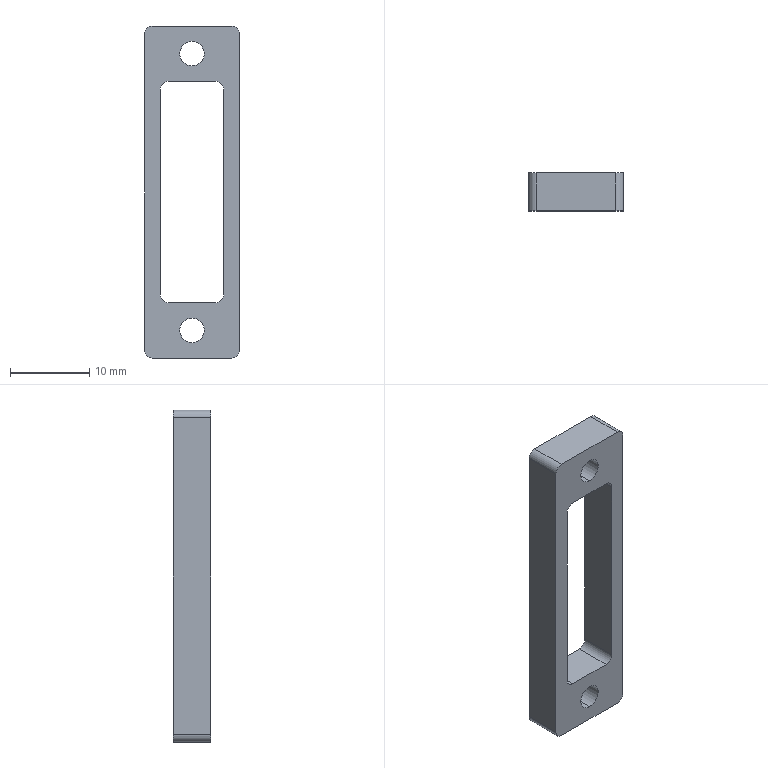Part | SolidWorks | features Extrusion 1, Fillet 1 | 1 solid | 22 faces | box 12 x 4.8 x 42 mm | volume 1272 mm3 | cylinder 12 | plane 10 | commonest cylinder face diameters 2 x8 3.1 x4
STEP:
#1=CARTESIAN_POINT('',(0.,4.8,-36.55));
#2=VERTEX_POINT('',#1);
#3=CARTESIAN_POINT('',(0.,4.8,-33.45));
#4=VERTEX_POINT('',#3);
#5=CARTESIAN_POINT('',(0.,4.8,-35.));
#6=DIRECTION('',(0.,1.,0.));
#7=DIRECTION('',(0.,0.,1.));
#8=AXIS2_PLACEMENT_3D('',#5,#6,#7);
#9=CIRCLE('',#8,1.55);
#10=EDGE_CURVE('',#2,#4,#9,.T.);
#11=ORIENTED_EDGE('',*,*,#10,.T.);
#12=CARTESIAN_POINT('',(0.,0.,-33.45));
#13=VERTEX_POINT('',#12);
#14=CARTESIAN_POINT('',(0.,4.8,-33.45));
#15=DIRECTION('',(0.,-1.,0.));
#16=VECTOR('',#15,1000.);
#17=LINE('',#14,#16);
#18=EDGE_CURVE('',#4,#13,#17,.T.);
#19=ORIENTED_EDGE('',*,*,#18,.T.);
#20=CARTESIAN_POINT('',(0.,0.,-36.55));
#21=VERTEX_POINT('',#20);
#22=CARTESIAN_POINT('',(0.,0.,-35.));
#23=DIRECTION('',(0.,1.,0.));
#24=DIRECTION('',(0.,0.,1.));
#25=AXIS2_PLACEMENT_3D('',#22,#23,#24);
#26=CIRCLE('',#25,1.55);
#27=EDGE_CURVE('',#21,#13,#26,.T.);
#28=ORIENTED_EDGE('',*,*,#27,.F.);
#29=CARTESIAN_POINT('',(0.,4.8,-36.55));
#30=DIRECTION('',(0.,-1.,0.));
#31=VECTOR('',#30,1000.);
#32=LINE('',#29,#31);
#33=EDGE_CURVE('',#2,#21,#32,.T.);
#34=ORIENTED_EDGE('',*,*,#33,.F.);
#35=EDGE_LOOP('',(#11,#19,#28,#34));
#36=FACE_OUTER_BOUND('',#35,.T.);
#37=CARTESIAN_POINT('',(0.,4.8,-35.));
#38=DIRECTION('',(0.,-1.,0.));
#39=DIRECTION('',(0.,0.,-1.));
#40=AXIS2_PLACEMENT_3D('',#37,#38,#39);
#41=CYLINDRICAL_SURFACE('',#40,1.55);
#42=ADVANCED_FACE('',(#36),#41,.F.);
#43=CARTESIAN_POINT('',(0.,4.8,-1.55));
#44=VERTEX_POINT('',#43);
#45=CARTESIAN_POINT('',(0.,4.8,1.55));
#46=VERTEX_POINT('',#45);
#47=CARTESIAN_POINT('',(0.,4.8,0.));
#48=DIRECTION('',(0.,1.,0.));
#49=DIRECTION('',(0.,0.,1.));
#50=AXIS2_PLACEMENT_3D('',#47,#48,#49);
#51=CIRCLE('',#50,1.55);
#52=EDGE_CURVE('',#44,#46,#51,.T.);
#53=ORIENTED_EDGE('',*,*,#52,.T.);
#54=CARTESIAN_POINT('',(0.,0.,1.55));
#55=VERTEX_POINT('',#54);
#56=CARTESIAN_POINT('',(0.,4.8,1.55));
#57=DIRECTION('',(0.,-1.,0.));
#58=VECTOR('',#57,1000.);
#59=LINE('',#56,#58);
#60=EDGE_CURVE('',#46,#55,#59,.T.);
#61=ORIENTED_EDGE('',*,*,#60,.T.);
#62=CARTESIAN_POINT('',(0.,0.,-1.55));
#63=VERTEX_POINT('',#62);
#64=CARTESIAN_POINT('',(0.,0.,0.));
#65=DIRECTION('',(0.,1.,0.));
#66=DIRECTION('',(0.,0.,1.));
#67=AXIS2_PLACEMENT_3D('',#64,#65,#66);
#68=CIRCLE('',#67,1.55);
#69=EDGE_CURVE('',#63,#55,#68,.T.);
#70=ORIENTED_EDGE('',*,*,#69,.F.);
#71=CARTESIAN_POINT('',(0.,4.8,-1.55));
#72=DIRECTION('',(0.,-1.,0.));
#73=VECTOR('',#72,1000.);
#74=LINE('',#71,#73);
#75=EDGE_CURVE('',#44,#63,#74,.T.);
#76=ORIENTED_EDGE('',*,*,#75,.F.);
#77=EDGE_LOOP('',(#53,#61,#70,#76));
#78=FACE_OUTER_BOUND('',#77,.T.);
#79=CARTESIAN_POINT('',(0.,4.8,0.));
#80=DIRECTION('',(0.,-1.,0.));
#81=DIRECTION('',(0.,0.,-1.));
#82=AXIS2_PLACEMENT_3D('',#79,#80,#81);
#83=CYLINDRICAL_SURFACE('',#82,1.55);
#84=ADVANCED_FACE('',(#78),#83,.F.);
#85=CARTESIAN_POINT('',(-4.,4.8,-30.5));
#86=VERTEX_POINT('',#85);
#87=CARTESIAN_POINT('',(-4.,4.8,-4.5));
#88=VERTEX_POINT('',#87);
#89=CARTESIAN_POINT('',(-4.,4.8,0.));
#90=DIRECTION('',(0.,0.,1.));
#91=VECTOR('',#90,1000.);
#92=LINE('',#89,#91);
#93=EDGE_CURVE('',#86,#88,#92,.T.);
#94=ORIENTED_EDGE('',*,*,#93,.T.);
#95=CARTESIAN_POINT('',(-4.,0.,-4.5));
#96=VERTEX_POINT('',#95);
#97=CARTESIAN_POINT('',(-4.,0.,-4.5));
#98=DIRECTION('',(0.,-1.,0.));
#99=VECTOR('',#98,1000.);
#100=LINE('',#97,#99);
#101=EDGE_CURVE('',#88,#96,#100,.T.);
#102=ORIENTED_EDGE('',*,*,#101,.T.);
#103=CARTESIAN_POINT('',(-4.,0.,-30.5));
#104=VERTEX_POINT('',#103);
#105=CARTESIAN_POINT('',(-4.,0.,0.));
#106=DIRECTION('',(0.,0.,1.));
#107=VECTOR('',#106,1000.);
#108=LINE('',#105,#107);
#109=EDGE_CURVE('',#104,#96,#108,.T.);
#110=ORIENTED_EDGE('',*,*,#109,.F.);
#111=CARTESIAN_POINT('',(-4.,4.8,-30.5));
#112=DIRECTION('',(0.,1.,0.));
#113=VECTOR('',#112,1000.);
#114=LINE('',#111,#113);
#115=EDGE_CURVE('',#104,#86,#114,.T.);
#116=ORIENTED_EDGE('',*,*,#115,.T.);
#117=EDGE_LOOP('',(#94,#102,#110,#116));
#118=FACE_OUTER_BOUND('',#117,.T.);
#119=CARTESIAN_POINT('',(-4.,4.8,0.));
#120=DIRECTION('',(1.,0.,0.));
#121=DIRECTION('',(0.,0.,-1.));
#122=AXIS2_PLACEMENT_3D('',#119,#120,#121);
#123=PLANE('',#122);
#124=ADVANCED_FACE('',(#118),#123,.T.);
#125=CARTESIAN_POINT('',(-3.,0.,-31.5));
#126=VERTEX_POINT('',#125);
#127=CARTESIAN_POINT('',(3.,0.,-31.5));
#128=VERTEX_POINT('',#127);
#129=CARTESIAN_POINT('',(0.,0.,-31.5));
#130=DIRECTION('',(1.,0.,0.));
#131=VECTOR('',#130,1000.);
#132=LINE('',#129,#131);
#133=EDGE_CURVE('',#126,#128,#132,.T.);
#134=ORIENTED_EDGE('',*,*,#133,.T.);
#135=CARTESIAN_POINT('',(3.,4.8,-31.5));
#136=VERTEX_POINT('',#135);
#137=CARTESIAN_POINT('',(3.,4.8,-31.5));
#138=DIRECTION('',(0.,1.,0.));
#139=VECTOR('',#138,1000.);
#140=LINE('',#137,#139);
#141=EDGE_CURVE('',#128,#136,#140,.T.);
#142=ORIENTED_EDGE('',*,*,#141,.T.);
#143=CARTESIAN_POINT('',(-3.,4.8,-31.5));
#144=VERTEX_POINT('',#143);
#145=CARTESIAN_POINT('',(0.,4.8,-31.5));
#146=DIRECTION('',(1.,0.,0.));
#147=VECTOR('',#146,1000.);
#148=LINE('',#145,#147);
#149=EDGE_CURVE('',#144,#136,#148,.T.);
#150=ORIENTED_EDGE('',*,*,#149,.F.);
#151=CARTESIAN_POINT('',(-3.,4.8,-31.5));
#152=DIRECTION('',(0.,-1.,0.));
#153=VECTOR('',#152,1000.);
#154=LINE('',#151,#153);
#155=EDGE_CURVE('',#144,#126,#154,.T.);
#156=ORIENTED_EDGE('',*,*,#155,.T.);
#157=EDGE_LOOP('',(#134,#142,#150,#156));
#158=FACE_OUTER_BOUND('',#157,.T.);
#159=CARTESIAN_POINT('',(0.,4.8,-31.5));
#160=DIRECTION('',(0.,0.,-1.));
#161=DIRECTION('',(-1.,0.,0.));
#162=AXIS2_PLACEMENT_3D('',#159,#160,#161);
#163=PLANE('',#162);
#164=ADVANCED_FACE('',(#158),#163,.F.);
#165=CARTESIAN_POINT('',(4.,0.,-30.5));
#166=VERTEX_POINT('',#165);
#167=CARTESIAN_POINT('',(4.,0.,-4.5));
#168=VERTEX_POINT('',#167);
#169=CARTESIAN_POINT('',(4.,0.,0.));
#170=DIRECTION('',(0.,0.,1.));
#171=VECTOR('',#170,1000.);
#172=LINE('',#169,#171);
#173=EDGE_CURVE('',#166,#168,#172,.T.);
#174=ORIENTED_EDGE('',*,*,#173,.T.);
#175=CARTESIAN_POINT('',(4.,4.8,-4.5));
#176=VERTEX_POINT('',#175);
#177=CARTESIAN_POINT('',(4.,4.8,-4.5));
#178=DIRECTION('',(0.,1.,0.));
#179=VECTOR('',#178,1000.);
#180=LINE('',#177,#179);
#181=EDGE_CURVE('',#168,#176,#180,.T.);
#182=ORIENTED_EDGE('',*,*,#181,.T.);
#183=CARTESIAN_POINT('',(4.,4.8,-30.5));
#184=VERTEX_POINT('',#183);
#185=CARTESIAN_POINT('',(4.,4.8,0.));
#186=DIRECTION('',(0.,0.,1.));
#187=VECTOR('',#186,1000.);
#188=LINE('',#185,#187);
#189=EDGE_CURVE('',#184,#176,#188,.T.);
#190=ORIENTED_EDGE('',*,*,#189,.F.);
#191=CARTESIAN_POINT('',(4.,0.,-30.5));
#192=DIRECTION('',(0.,-1.,0.));
#193=VECTOR('',#192,1000.);
#194=LINE('',#191,#193);
#195=EDGE_CURVE('',#184,#166,#194,.T.);
#196=ORIENTED_EDGE('',*,*,#195,.T.);
#197=EDGE_LOOP('',(#174,#182,#190,#196));
#198=FACE_OUTER_BOUND('',#197,.T.);
#199=CARTESIAN_POINT('',(4.,4.8,0.));
#200=DIRECTION('',(1.,0.,0.));
#201=DIRECTION('',(0.,0.,-1.));
#202=AXIS2_PLACEMENT_3D('',#199,#200,#201);
#203=PLANE('',#202);
#204=ADVANCED_FACE('',(#198),#203,.F.);
#205=CARTESIAN_POINT('',(6.,0.,-37.5));
#206=VERTEX_POINT('',#205);
#207=CARTESIAN_POINT('',(6.,0.,2.5));
#208=VERTEX_POINT('',#207);
#209=CARTESIAN_POINT('',(6.,0.,0.));
#210=DIRECTION('',(0.,0.,1.));
#211=VECTOR('',#210,1000.);
#212=LINE('',#209,#211);
#213=EDGE_CURVE('',#206,#208,#212,.T.);
#214=ORIENTED_EDGE('',*,*,#213,.F.);
#215=CARTESIAN_POINT('',(6.,4.8,-37.5));
#216=VERTEX_POINT('',#215);
#217=CARTESIAN_POINT('',(6.,4.8,-37.5));
#218=DIRECTION('',(0.,1.,0.));
#219=VECTOR('',#218,1000.);
#220=LINE('',#217,#219);
#221=EDGE_CURVE('',#206,#216,#220,.T.);
#222=ORIENTED_EDGE('',*,*,#221,.T.);
#223=CARTESIAN_POINT('',(6.,4.8,2.5));
#224=VERTEX_POINT('',#223);
#225=CARTESIAN_POINT('',(6.,4.8,0.));
#226=DIRECTION('',(0.,0.,1.));
#227=VECTOR('',#226,1000.);
#228=LINE('',#225,#227);
#229=EDGE_CURVE('',#216,#224,#228,.T.);
#230=ORIENTED_EDGE('',*,*,#229,.T.);
#231=CARTESIAN_POINT('',(6.,0.,2.5));
#232=DIRECTION('',(0.,-1.,0.));
#233=VECTOR('',#232,1000.);
#234=LINE('',#231,#233);
#235=EDGE_CURVE('',#224,#208,#234,.T.);
#236=ORIENTED_EDGE('',*,*,#235,.T.);
#237=EDGE_LOOP('',(#214,#222,#230,#236));
#238=FACE_OUTER_BOUND('',#237,.T.);
#239=CARTESIAN_POINT('',(6.,4.8,0.));
#240=DIRECTION('',(1.,0.,0.));
#241=DIRECTION('',(0.,0.,-1.));
#242=AXIS2_PLACEMENT_3D('',#239,#240,#241);
#243=PLANE('',#242);
#244=ADVANCED_FACE('',(#238),#243,.T.);
#245=CARTESIAN_POINT('',(-5.,0.,-38.5));
#246=VERTEX_POINT('',#245);
#247=CARTESIAN_POINT('',(5.,0.,-38.5));
#248=VERTEX_POINT('',#247);
#249=CARTESIAN_POINT('',(0.,0.,-38.5));
#250=DIRECTION('',(1.,0.,0.));
#251=VECTOR('',#250,1000.);
#252=LINE('',#249,#251);
#253=EDGE_CURVE('',#246,#248,#252,.T.);
#254=ORIENTED_EDGE('',*,*,#253,.F.);
#255=CARTESIAN_POINT('',(-5.,4.8,-38.5));
#256=VERTEX_POINT('',#255);
#257=CARTESIAN_POINT('',(-5.,4.8,-38.5));
#258=DIRECTION('',(0.,1.,0.));
#259=VECTOR('',#258,1000.);
#260=LINE('',#257,#259);
#261=EDGE_CURVE('',#246,#256,#260,.T.);
#262=ORIENTED_EDGE('',*,*,#261,.T.);
#263=CARTESIAN_POINT('',(5.,4.8,-38.5));
#264=VERTEX_POINT('',#263);
#265=CARTESIAN_POINT('',(0.,4.8,-38.5));
#266=DIRECTION('',(1.,0.,0.));
#267=VECTOR('',#266,1000.);
#268=LINE('',#265,#267);
#269=EDGE_CURVE('',#256,#264,#268,.T.);
#270=ORIENTED_EDGE('',*,*,#269,.T.);
#271=CARTESIAN_POINT('',(5.,4.8,-38.5));
#272=DIRECTION('',(0.,-1.,0.));
#273=VECTOR('',#272,1000.);
#274=LINE('',#271,#273);
#275=EDGE_CURVE('',#264,#248,#274,.T.);
#276=ORIENTED_EDGE('',*,*,#275,.T.);
#277=EDGE_LOOP('',(#254,#262,#270,#276));
#278=FACE_OUTER_BOUND('',#277,.T.);
#279=CARTESIAN_POINT('',(0.,4.8,-38.5));
#280=DIRECTION('',(0.,0.,-1.));
#281=DIRECTION('',(-1.,0.,0.));
#282=AXIS2_PLACEMENT_3D('',#279,#280,#281);
#283=PLANE('',#282);
#284=ADVANCED_FACE('',(#278),#283,.T.);
#285=CARTESIAN_POINT('',(-6.,4.8,-37.5));
#286=VERTEX_POINT('',#285);
#287=CARTESIAN_POINT('',(-6.,4.8,2.5));
#288=VERTEX_POINT('',#287);
#289=CARTESIAN_POINT('',(-6.,4.8,0.));
#290=DIRECTION('',(0.,0.,1.));
#291=VECTOR('',#290,1000.);
#292=LINE('',#289,#291);
#293=EDGE_CURVE('',#286,#288,#292,.T.);
#294=ORIENTED_EDGE('',*,*,#293,.F.);
#295=CARTESIAN_POINT('',(-6.,0.,-37.5));
#296=VERTEX_POINT('',#295);
#297=CARTESIAN_POINT('',(-6.,0.,-37.5));
#298=DIRECTION('',(0.,-1.,0.));
#299=VECTOR('',#298,1000.);
#300=LINE('',#297,#299);
#301=EDGE_CURVE('',#286,#296,#300,.T.);
#302=ORIENTED_EDGE('',*,*,#301,.T.);
#303=CARTESIAN_POINT('',(-6.,0.,2.5));
#304=VERTEX_POINT('',#303);
#305=CARTESIAN_POINT('',(-6.,0.,0.));
#306=DIRECTION('',(0.,0.,1.));
#307=VECTOR('',#306,1000.);
#308=LINE('',#305,#307);
#309=EDGE_CURVE('',#296,#304,#308,.T.);
#310=ORIENTED_EDGE('',*,*,#309,.T.);
#311=CARTESIAN_POINT('',(-6.,4.8,2.5));
#312=DIRECTION('',(0.,1.,0.));
#313=VECTOR('',#312,1000.);
#314=LINE('',#311,#313);
#315=EDGE_CURVE('',#304,#288,#314,.T.);
#316=ORIENTED_EDGE('',*,*,#315,.T.);
#317=EDGE_LOOP('',(#294,#302,#310,#316));
#318=FACE_OUTER_BOUND('',#317,.T.);
#319=CARTESIAN_POINT('',(-6.,4.8,0.));
#320=DIRECTION('',(1.,0.,0.));
#321=DIRECTION('',(0.,0.,-1.));
#322=AXIS2_PLACEMENT_3D('',#319,#320,#321);
#323=PLANE('',#322);
#324=ADVANCED_FACE('',(#318),#323,.F.);
#325=ORIENTED_EDGE('',*,*,#60,.F.);
#326=CARTESIAN_POINT('',(0.,4.8,0.));
#327=DIRECTION('',(0.,1.,0.));
#328=DIRECTION('',(0.,0.,1.));
#329=AXIS2_PLACEMENT_3D('',#326,#327,#328);
#330=CIRCLE('',#329,1.55);
#331=EDGE_CURVE('',#46,#44,#330,.T.);
#332=ORIENTED_EDGE('',*,*,#331,.T.);
#333=ORIENTED_EDGE('',*,*,#75,.T.);
#334=CARTESIAN_POINT('',(0.,0.,0.));
#335=DIRECTION('',(0.,1.,0.));
#336=DIRECTION('',(0.,0.,1.));
#337=AXIS2_PLACEMENT_3D('',#334,#335,#336);
#338=CIRCLE('',#337,1.55);
#339=EDGE_CURVE('',#55,#63,#338,.T.);
#340=ORIENTED_EDGE('',*,*,#339,.F.);
#341=EDGE_LOOP('',(#325,#332,#333,#340));
#342=FACE_OUTER_BOUND('',#341,.T.);
#343=CARTESIAN_POINT('',(0.,4.8,0.));
#344=DIRECTION('',(0.,-1.,0.));
#345=DIRECTION('',(0.,0.,-1.));
#346=AXIS2_PLACEMENT_3D('',#343,#344,#345);
#347=CYLINDRICAL_SURFACE('',#346,1.55);
#348=ADVANCED_FACE('',(#342),#347,.F.);
#349=CARTESIAN_POINT('',(-3.,0.,-3.5));
#350=VERTEX_POINT('',#349);
#351=CARTESIAN_POINT('',(3.,0.,-3.5));
#352=VERTEX_POINT('',#351);
#353=CARTESIAN_POINT('',(0.,0.,-3.5));
#354=DIRECTION('',(1.,0.,0.));
#355=VECTOR('',#354,1000.);
#356=LINE('',#353,#355);
#357=EDGE_CURVE('',#350,#352,#356,.T.);
#358=ORIENTED_EDGE('',*,*,#357,.F.);
#359=CARTESIAN_POINT('',(-3.,4.8,-3.5));
#360=VERTEX_POINT('',#359);
#361=CARTESIAN_POINT('',(-3.,4.8,-3.5));
#362=DIRECTION('',(0.,1.,0.));
#363=VECTOR('',#362,1000.);
#364=LINE('',#361,#363);
#365=EDGE_CURVE('',#350,#360,#364,.T.);
#366=ORIENTED_EDGE('',*,*,#365,.T.);
#367=CARTESIAN_POINT('',(3.,4.8,-3.5));
#368=VERTEX_POINT('',#367);
#369=CARTESIAN_POINT('',(0.,4.8,-3.5));
#370=DIRECTION('',(1.,0.,0.));
#371=VECTOR('',#370,1000.);
#372=LINE('',#369,#371);
#373=EDGE_CURVE('',#360,#368,#372,.T.);
#374=ORIENTED_EDGE('',*,*,#373,.T.);
#375=CARTESIAN_POINT('',(3.,4.8,-3.5));
#376=DIRECTION('',(0.,-1.,0.));
#377=VECTOR('',#376,1000.);
#378=LINE('',#375,#377);
#379=EDGE_CURVE('',#368,#352,#378,.T.);
#380=ORIENTED_EDGE('',*,*,#379,.T.);
#381=EDGE_LOOP('',(#358,#366,#374,#380));
#382=FACE_OUTER_BOUND('',#381,.T.);
#383=CARTESIAN_POINT('',(0.,4.8,-3.5));
#384=DIRECTION('',(0.,0.,-1.));
#385=DIRECTION('',(-1.,0.,0.));
#386=AXIS2_PLACEMENT_3D('',#383,#384,#385);
#387=PLANE('',#386);
#388=ADVANCED_FACE('',(#382),#387,.T.);
#389=CARTESIAN_POINT('',(-5.,0.,3.5));
#390=VERTEX_POINT('',#389);
#391=CARTESIAN_POINT('',(5.,0.,3.5));
#392=VERTEX_POINT('',#391);
#393=CARTESIAN_POINT('',(0.,0.,3.5));
#394=DIRECTION('',(1.,0.,0.));
#395=VECTOR('',#394,1000.);
#396=LINE('',#393,#395);
#397=EDGE_CURVE('',#390,#392,#396,.T.);
#398=ORIENTED_EDGE('',*,*,#397,.T.);
#399=CARTESIAN_POINT('',(5.,4.8,3.5));
#400=VERTEX_POINT('',#399);
#401=CARTESIAN_POINT('',(5.,4.8,3.5));
#402=DIRECTION('',(0.,1.,0.));
#403=VECTOR('',#402,1000.);
#404=LINE('',#401,#403);
#405=EDGE_CURVE('',#392,#400,#404,.T.);
#406=ORIENTED_EDGE('',*,*,#405,.T.);
#407=CARTESIAN_POINT('',(-5.,4.8,3.5));
#408=VERTEX_POINT('',#407);
#409=CARTESIAN_POINT('',(0.,4.8,3.5));
#410=DIRECTION('',(1.,0.,0.));
#411=VECTOR('',#410,1000.);
#412=LINE('',#409,#411);
#413=EDGE_CURVE('',#408,#400,#412,.T.);
#414=ORIENTED_EDGE('',*,*,#413,.F.);
#415=CARTESIAN_POINT('',(-5.,4.8,3.5));
#416=DIRECTION('',(0.,-1.,0.));
#417=VECTOR('',#416,1000.);
#418=LINE('',#415,#417);
#419=EDGE_CURVE('',#408,#390,#418,.T.);
#420=ORIENTED_EDGE('',*,*,#419,.T.);
#421=EDGE_LOOP('',(#398,#406,#414,#420));
#422=FACE_OUTER_BOUND('',#421,.T.);
#423=CARTESIAN_POINT('',(0.,4.8,3.5));
#424=DIRECTION('',(0.,0.,-1.));
#425=DIRECTION('',(-1.,0.,0.));
#426=AXIS2_PLACEMENT_3D('',#423,#424,#425);
#427=PLANE('',#426);
#428=ADVANCED_FACE('',(#422),#427,.F.);
#429=ORIENTED_EDGE('',*,*,#18,.F.);
#430=CARTESIAN_POINT('',(0.,4.8,-35.));
#431=DIRECTION('',(0.,1.,0.));
#432=DIRECTION('',(0.,0.,1.));
#433=AXIS2_PLACEMENT_3D('',#430,#431,#432);
#434=CIRCLE('',#433,1.55);
#435=EDGE_CURVE('',#4,#2,#434,.T.);
#436=ORIENTED_EDGE('',*,*,#435,.T.);
#437=ORIENTED_EDGE('',*,*,#33,.T.);
#438=CARTESIAN_POINT('',(0.,0.,-35.));
#439=DIRECTION('',(0.,1.,0.));
#440=DIRECTION('',(0.,0.,1.));
#441=AXIS2_PLACEMENT_3D('',#438,#439,#440);
#442=CIRCLE('',#441,1.55);
#443=EDGE_CURVE('',#13,#21,#442,.T.);
#444=ORIENTED_EDGE('',*,*,#443,.F.);
#445=EDGE_LOOP('',(#429,#436,#437,#444));
#446=FACE_OUTER_BOUND('',#445,.T.);
#447=CARTESIAN_POINT('',(0.,4.8,-35.));
#448=DIRECTION('',(0.,-1.,0.));
#449=DIRECTION('',(0.,0.,-1.));
#450=AXIS2_PLACEMENT_3D('',#447,#448,#449);
#451=CYLINDRICAL_SURFACE('',#450,1.55);
#452=ADVANCED_FACE('',(#446),#451,.F.);
#453=ORIENTED_EDGE('',*,*,#269,.F.);
#454=CARTESIAN_POINT('',(-5.,4.8,-37.5));
#455=DIRECTION('',(0.,1.,0.));
#456=DIRECTION('',(0.,0.,1.));
#457=AXIS2_PLACEMENT_3D('',#454,#455,#456);
#458=CIRCLE('',#457,1.);
#459=EDGE_CURVE('',#256,#286,#458,.T.);
#460=ORIENTED_EDGE('',*,*,#459,.T.);
#461=ORIENTED_EDGE('',*,*,#293,.T.);
#462=CARTESIAN_POINT('',(-5.,4.8,2.5));
#463=DIRECTION('',(0.,1.,0.));
#464=DIRECTION('',(0.,0.,1.));
#465=AXIS2_PLACEMENT_3D('',#462,#463,#464);
#466=CIRCLE('',#465,1.);
#467=EDGE_CURVE('',#288,#408,#466,.T.);
#468=ORIENTED_EDGE('',*,*,#467,.T.);
#469=ORIENTED_EDGE('',*,*,#413,.T.);
#470=CARTESIAN_POINT('',(5.,4.8,2.5));
#471=DIRECTION('',(0.,1.,0.));
#472=DIRECTION('',(0.,0.,1.));
#473=AXIS2_PLACEMENT_3D('',#470,#471,#472);
#474=CIRCLE('',#473,1.);
#475=EDGE_CURVE('',#400,#224,#474,.T.);
#476=ORIENTED_EDGE('',*,*,#475,.T.);
#477=ORIENTED_EDGE('',*,*,#229,.F.);
#478=CARTESIAN_POINT('',(5.,4.8,-37.5));
#479=DIRECTION('',(0.,1.,0.));
#480=DIRECTION('',(0.,0.,1.));
#481=AXIS2_PLACEMENT_3D('',#478,#479,#480);
#482=CIRCLE('',#481,1.);
#483=EDGE_CURVE('',#216,#264,#482,.T.);
#484=ORIENTED_EDGE('',*,*,#483,.T.);
#485=EDGE_LOOP('',(#453,#460,#461,#468,#469,#476,#477,#484));
#486=FACE_OUTER_BOUND('',#485,.T.);
#487=ORIENTED_EDGE('',*,*,#93,.F.);
#488=CARTESIAN_POINT('',(-3.,4.8,-30.5));
#489=DIRECTION('',(0.,-1.,0.));
#490=DIRECTION('',(0.,0.,1.));
#491=AXIS2_PLACEMENT_3D('',#488,#489,#490);
#492=CIRCLE('',#491,1.);
#493=EDGE_CURVE('',#86,#144,#492,.T.);
#494=ORIENTED_EDGE('',*,*,#493,.T.);
#495=ORIENTED_EDGE('',*,*,#149,.T.);
#496=CARTESIAN_POINT('',(3.,4.8,-30.5));
#497=DIRECTION('',(0.,-1.,0.));
#498=DIRECTION('',(0.,0.,1.));
#499=AXIS2_PLACEMENT_3D('',#496,#497,#498);
#500=CIRCLE('',#499,1.);
#501=EDGE_CURVE('',#136,#184,#500,.T.);
#502=ORIENTED_EDGE('',*,*,#501,.T.);
#503=ORIENTED_EDGE('',*,*,#189,.T.);
#504=CARTESIAN_POINT('',(3.,4.8,-4.5));
#505=DIRECTION('',(0.,-1.,0.));
#506=DIRECTION('',(0.,0.,1.));
#507=AXIS2_PLACEMENT_3D('',#504,#505,#506);
#508=CIRCLE('',#507,1.);
#509=EDGE_CURVE('',#176,#368,#508,.T.);
#510=ORIENTED_EDGE('',*,*,#509,.T.);
#511=ORIENTED_EDGE('',*,*,#373,.F.);
#512=CARTESIAN_POINT('',(-3.,4.8,-4.5));
#513=DIRECTION('',(0.,-1.,0.));
#514=DIRECTION('',(0.,0.,1.));
#515=AXIS2_PLACEMENT_3D('',#512,#513,#514);
#516=CIRCLE('',#515,1.);
#517=EDGE_CURVE('',#360,#88,#516,.T.);
#518=ORIENTED_EDGE('',*,*,#517,.T.);
#519=EDGE_LOOP('',(#487,#494,#495,#502,#503,#510,#511,#518));
#520=FACE_BOUND('',#519,.T.);
#521=ORIENTED_EDGE('',*,*,#52,.F.);
#522=ORIENTED_EDGE('',*,*,#331,.F.);
#523=EDGE_LOOP('',(#521,#522));
#524=FACE_BOUND('',#523,.T.);
#525=ORIENTED_EDGE('',*,*,#10,.F.);
#526=ORIENTED_EDGE('',*,*,#435,.F.);
#527=EDGE_LOOP('',(#525,#526));
#528=FACE_BOUND('',#527,.T.);
#529=CARTESIAN_POINT('',(0.,4.8,0.));
#530=DIRECTION('',(0.,1.,0.));
#531=DIRECTION('',(0.,0.,1.));
#532=AXIS2_PLACEMENT_3D('',#529,#530,#531);
#533=PLANE('',#532);
#534=ADVANCED_FACE('',(#486,#520,#524,#528),#533,.T.);
#535=ORIENTED_EDGE('',*,*,#309,.F.);
#536=CARTESIAN_POINT('',(-5.,0.,-37.5));
#537=DIRECTION('',(0.,-1.,0.));
#538=DIRECTION('',(0.,0.,1.));
#539=AXIS2_PLACEMENT_3D('',#536,#537,#538);
#540=CIRCLE('',#539,1.);
#541=EDGE_CURVE('',#296,#246,#540,.T.);
#542=ORIENTED_EDGE('',*,*,#541,.T.);
#543=ORIENTED_EDGE('',*,*,#253,.T.);
#544=CARTESIAN_POINT('',(5.,0.,-37.5));
#545=DIRECTION('',(0.,-1.,0.));
#546=DIRECTION('',(0.,0.,1.));
#547=AXIS2_PLACEMENT_3D('',#544,#545,#546);
#548=CIRCLE('',#547,1.);
#549=EDGE_CURVE('',#248,#206,#548,.T.);
#550=ORIENTED_EDGE('',*,*,#549,.T.);
#551=ORIENTED_EDGE('',*,*,#213,.T.);
#552=CARTESIAN_POINT('',(5.,0.,2.5));
#553=DIRECTION('',(0.,-1.,0.));
#554=DIRECTION('',(0.,0.,1.));
#555=AXIS2_PLACEMENT_3D('',#552,#553,#554);
#556=CIRCLE('',#555,1.);
#557=EDGE_CURVE('',#208,#392,#556,.T.);
#558=ORIENTED_EDGE('',*,*,#557,.T.);
#559=ORIENTED_EDGE('',*,*,#397,.F.);
#560=CARTESIAN_POINT('',(-5.,0.,2.5));
#561=DIRECTION('',(0.,-1.,0.));
#562=DIRECTION('',(0.,0.,1.));
#563=AXIS2_PLACEMENT_3D('',#560,#561,#562);
#564=CIRCLE('',#563,1.);
#565=EDGE_CURVE('',#390,#304,#564,.T.);
#566=ORIENTED_EDGE('',*,*,#565,.T.);
#567=EDGE_LOOP('',(#535,#542,#543,#550,#551,#558,#559,#566));
#568=FACE_OUTER_BOUND('',#567,.T.);
#569=ORIENTED_EDGE('',*,*,#133,.F.);
#570=CARTESIAN_POINT('',(-3.,0.,-30.5));
#571=DIRECTION('',(0.,1.,0.));
#572=DIRECTION('',(0.,0.,1.));
#573=AXIS2_PLACEMENT_3D('',#570,#571,#572);
#574=CIRCLE('',#573,1.);
#575=EDGE_CURVE('',#126,#104,#574,.T.);
#576=ORIENTED_EDGE('',*,*,#575,.T.);
#577=ORIENTED_EDGE('',*,*,#109,.T.);
#578=CARTESIAN_POINT('',(-3.,0.,-4.5));
#579=DIRECTION('',(0.,1.,0.));
#580=DIRECTION('',(0.,0.,1.));
#581=AXIS2_PLACEMENT_3D('',#578,#579,#580);
#582=CIRCLE('',#581,1.);
#583=EDGE_CURVE('',#96,#350,#582,.T.);
#584=ORIENTED_EDGE('',*,*,#583,.T.);
#585=ORIENTED_EDGE('',*,*,#357,.T.);
#586=CARTESIAN_POINT('',(3.,0.,-4.5));
#587=DIRECTION('',(0.,1.,0.));
#588=DIRECTION('',(0.,0.,1.));
#589=AXIS2_PLACEMENT_3D('',#586,#587,#588);
#590=CIRCLE('',#589,1.);
#591=EDGE_CURVE('',#352,#168,#590,.T.);
#592=ORIENTED_EDGE('',*,*,#591,.T.);
#593=ORIENTED_EDGE('',*,*,#173,.F.);
#594=CARTESIAN_POINT('',(3.,0.,-30.5));
#595=DIRECTION('',(0.,1.,0.));
#596=DIRECTION('',(0.,0.,1.));
#597=AXIS2_PLACEMENT_3D('',#594,#595,#596);
#598=CIRCLE('',#597,1.);
#599=EDGE_CURVE('',#166,#128,#598,.T.);
#600=ORIENTED_EDGE('',*,*,#599,.T.);
#601=EDGE_LOOP('',(#569,#576,#577,#584,#585,#592,#593,#600));
#602=FACE_BOUND('',#601,.T.);
#603=ORIENTED_EDGE('',*,*,#69,.T.);
#604=ORIENTED_EDGE('',*,*,#339,.T.);
#605=EDGE_LOOP('',(#603,#604));
#606=FACE_BOUND('',#605,.T.);
#607=ORIENTED_EDGE('',*,*,#27,.T.);
#608=ORIENTED_EDGE('',*,*,#443,.T.);
#609=EDGE_LOOP('',(#607,#608));
#610=FACE_BOUND('',#609,.T.);
#611=CARTESIAN_POINT('',(0.,0.,0.));
#612=DIRECTION('',(0.,1.,0.));
#613=DIRECTION('',(0.,0.,1.));
#614=AXIS2_PLACEMENT_3D('',#611,#612,#613);
#615=PLANE('',#614);
#616=ADVANCED_FACE('',(#568,#602,#606,#610),#615,.F.);
#617=ORIENTED_EDGE('',*,*,#517,.F.);
#618=ORIENTED_EDGE('',*,*,#365,.F.);
#619=ORIENTED_EDGE('',*,*,#583,.F.);
#620=ORIENTED_EDGE('',*,*,#101,.F.);
#621=EDGE_LOOP('',(#617,#618,#619,#620));
#622=FACE_OUTER_BOUND('',#621,.T.);
#623=CARTESIAN_POINT('',(-3.,4.8,-4.5));
#624=DIRECTION('',(0.,1.,0.));
#625=DIRECTION('',(0.,0.,1.));
#626=AXIS2_PLACEMENT_3D('',#623,#624,#625);
#627=CYLINDRICAL_SURFACE('',#626,1.);
#628=ADVANCED_FACE('',(#622),#627,.F.);
#629=ORIENTED_EDGE('',*,*,#509,.F.);
#630=ORIENTED_EDGE('',*,*,#181,.F.);
#631=ORIENTED_EDGE('',*,*,#591,.F.);
#632=ORIENTED_EDGE('',*,*,#379,.F.);
#633=EDGE_LOOP('',(#629,#630,#631,#632));
#634=FACE_OUTER_BOUND('',#633,.T.);
#635=CARTESIAN_POINT('',(3.,4.8,-4.5));
#636=DIRECTION('',(0.,-1.,0.));
#637=DIRECTION('',(0.,0.,-1.));
#638=AXIS2_PLACEMENT_3D('',#635,#636,#637);
#639=CYLINDRICAL_SURFACE('',#638,1.);
#640=ADVANCED_FACE('',(#634),#639,.F.);
#641=ORIENTED_EDGE('',*,*,#501,.F.);
#642=ORIENTED_EDGE('',*,*,#141,.F.);
#643=ORIENTED_EDGE('',*,*,#599,.F.);
#644=ORIENTED_EDGE('',*,*,#195,.F.);
#645=EDGE_LOOP('',(#641,#642,#643,#644));
#646=FACE_OUTER_BOUND('',#645,.T.);
#647=CARTESIAN_POINT('',(3.,4.8,-30.5));
#648=DIRECTION('',(0.,1.,0.));
#649=DIRECTION('',(0.,0.,1.));
#650=AXIS2_PLACEMENT_3D('',#647,#648,#649);
#651=CYLINDRICAL_SURFACE('',#650,1.);
#652=ADVANCED_FACE('',(#646),#651,.F.);
#653=ORIENTED_EDGE('',*,*,#459,.F.);
#654=ORIENTED_EDGE('',*,*,#261,.F.);
#655=ORIENTED_EDGE('',*,*,#541,.F.);
#656=ORIENTED_EDGE('',*,*,#301,.F.);
#657=EDGE_LOOP('',(#653,#654,#655,#656));
#658=FACE_OUTER_BOUND('',#657,.T.);
#659=CARTESIAN_POINT('',(-5.,4.8,-37.5));
#660=DIRECTION('',(0.,1.,0.));
#661=DIRECTION('',(0.,0.,1.));
#662=AXIS2_PLACEMENT_3D('',#659,#660,#661);
#663=CYLINDRICAL_SURFACE('',#662,1.);
#664=ADVANCED_FACE('',(#658),#663,.T.);
#665=ORIENTED_EDGE('',*,*,#483,.F.);
#666=ORIENTED_EDGE('',*,*,#221,.F.);
#667=ORIENTED_EDGE('',*,*,#549,.F.);
#668=ORIENTED_EDGE('',*,*,#275,.F.);
#669=EDGE_LOOP('',(#665,#666,#667,#668));
#670=FACE_OUTER_BOUND('',#669,.T.);
#671=CARTESIAN_POINT('',(5.,4.8,-37.5));
#672=DIRECTION('',(0.,-1.,0.));
#673=DIRECTION('',(0.,0.,-1.));
#674=AXIS2_PLACEMENT_3D('',#671,#672,#673);
#675=CYLINDRICAL_SURFACE('',#674,1.);
#676=ADVANCED_FACE('',(#670),#675,.T.);
#677=ORIENTED_EDGE('',*,*,#493,.F.);
#678=ORIENTED_EDGE('',*,*,#115,.F.);
#679=ORIENTED_EDGE('',*,*,#575,.F.);
#680=ORIENTED_EDGE('',*,*,#155,.F.);
#681=EDGE_LOOP('',(#677,#678,#679,#680));
#682=FACE_OUTER_BOUND('',#681,.T.);
#683=CARTESIAN_POINT('',(-3.,4.8,-30.5));
#684=DIRECTION('',(0.,-1.,0.));
#685=DIRECTION('',(0.,0.,-1.));
#686=AXIS2_PLACEMENT_3D('',#683,#684,#685);
#687=CYLINDRICAL_SURFACE('',#686,1.);
#688=ADVANCED_FACE('',(#682),#687,.F.);
#689=ORIENTED_EDGE('',*,*,#475,.F.);
#690=ORIENTED_EDGE('',*,*,#405,.F.);
#691=ORIENTED_EDGE('',*,*,#557,.F.);
#692=ORIENTED_EDGE('',*,*,#235,.F.);
#693=EDGE_LOOP('',(#689,#690,#691,#692));
#694=FACE_OUTER_BOUND('',#693,.T.);
#695=CARTESIAN_POINT('',(5.,4.8,2.5));
#696=DIRECTION('',(0.,1.,0.));
#697=DIRECTION('',(0.,0.,1.));
#698=AXIS2_PLACEMENT_3D('',#695,#696,#697);
#699=CYLINDRICAL_SURFACE('',#698,1.);
#700=ADVANCED_FACE('',(#694),#699,.T.);
#701=ORIENTED_EDGE('',*,*,#467,.F.);
#702=ORIENTED_EDGE('',*,*,#315,.F.);
#703=ORIENTED_EDGE('',*,*,#565,.F.);
#704=ORIENTED_EDGE('',*,*,#419,.F.);
#705=EDGE_LOOP('',(#701,#702,#703,#704));
#706=FACE_OUTER_BOUND('',#705,.T.);
#707=CARTESIAN_POINT('',(-5.,4.8,2.5));
#708=DIRECTION('',(0.,-1.,0.));
#709=DIRECTION('',(0.,0.,-1.));
#710=AXIS2_PLACEMENT_3D('',#707,#708,#709);
#711=CYLINDRICAL_SURFACE('',#710,1.);
#712=ADVANCED_FACE('',(#706),#711,.T.);
#713=CLOSED_SHELL('',(#42,#84,#124,#164,#204,#244,#284,#324,#348,#388,#428,#452,#534,#616,#628,#640,#652,#664,#676,#688,#700,#712));
#714=MANIFOLD_SOLID_BREP('',#713);
#715=CARTESIAN_POINT('',(0.,0.,0.));
#716=DIRECTION('',(0.,0.,1.));
#717=DIRECTION('',(1.,0.,0.));
#718=AXIS2_PLACEMENT_3D('',#715,#716,#717);
#719=(LENGTH_UNIT()NAMED_UNIT(*)SI_UNIT(.MILLI.,.METRE.));
#720=UNCERTAINTY_MEASURE_WITH_UNIT(LENGTH_MEASURE(0.00001),#719,'','');
#721=(NAMED_UNIT(*)PLANE_ANGLE_UNIT()SI_UNIT($,.RADIAN.));
#722=(NAMED_UNIT(*)SI_UNIT($,.STERADIAN.)SOLID_ANGLE_UNIT());
#723=(GEOMETRIC_REPRESENTATION_CONTEXT(3)GLOBAL_UNCERTAINTY_ASSIGNED_CONTEXT((#720))GLOBAL_UNIT_ASSIGNED_CONTEXT((#719,#721,#722))REPRESENTATION_CONTEXT('',''));
#724=ADVANCED_BREP_SHAPE_REPRESENTATION('',(#714,#718),#723);